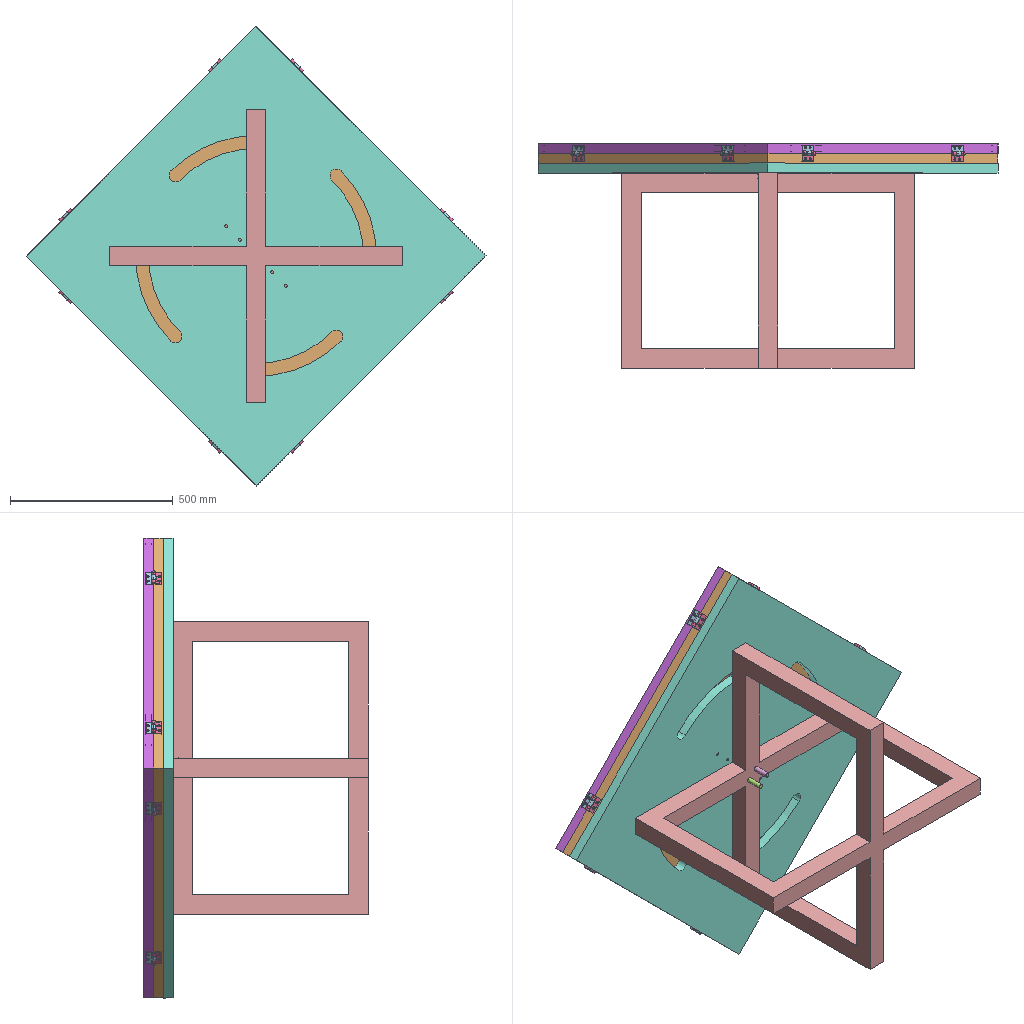Assembly | SolidWorks | 14 different items | 55 placed | box 1414 x 690 x 1414 mm
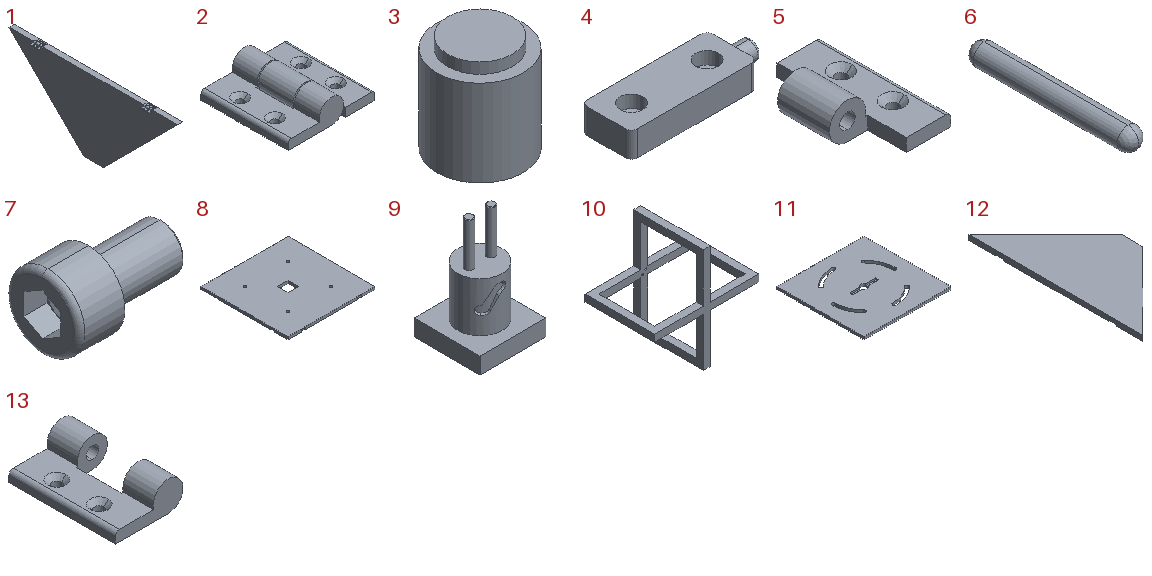Parts list (item | name | quantity | parent item | size | volume | features):
1 | (subassembly) | x4 | - | 55 x 1000 x 447 mm | 2719433 mm3 | -
2 | (subassembly) | x8 | in 1 | 50 x 50 x 14 mm | 16276 mm3 | -
3 | - | x4 | - | 40 x 40 x 45 mm | 53800 mm3 | features Extrusion 1, ICE 1
4 | - | x2 | - | 115 x 40 x 20 mm | 75193 mm3 | features Fillet 2, ICE 2, Extrusion 1
5 | - | x8 | in 2 | 32 x 50 x 14 mm | 6828 mm3 | features BaseBody 1
6 | - | x8 | in 2 | 6 x 46 x 6 mm | 1244 mm3 | features BaseBody 1
7 | - | x4 | - | 26 x 16 x 16 mm | 2933 mm3 | features Fillet 2, RevCut 2, Boss 1, Chamfer 1, Cut 1, Extrusion 1, LPattern 1
8 | - | x1 | - | 1000 x 1000 x 30 mm | 29440024 mm3 | features CirPattern 2, ICE 2, Extrusion 1, HoleWzd 1
9 | - | x1 | - | 120 x 120 x 200 mm | 904225 mm3 | features ICE 3, Chamfer 2, CirPattern 1, Emboss 1, Extrusion 1
10 | - | x1 | - | 900 x 600 x 900 mm | 19278601 mm3 | features ICE 2, Extrusion 1, HoleWzd 1
11 | - | x1 | - | 1000 x 1000 x 30 mm | 28197892 mm3 | features ICE 3, Extrusion 1, HoleWzd 1
12 | - | x4 | in 1 | 440 x 1000 x 30 mm | 2685666 mm3 | features Cut 1, Extrusion 1, HoleWzd 1, ICE 1, Shell 1
13 | - | x8 | in 2 | 32 x 50 x 14 mm | 8203 mm3 | features BaseBody 1
14 | cross recessed ctsk thread forming screw gb | x1 | - | - | - | -
Mates (type | each side: item.copy, entity, surface, feature):
In the top assembly
Concentric | 10.1 face cylinder Blind dowel hole 0 (size mm) | 9.1 face cylinder Boss-Extrude3 | 2 times
Concentric | 8.1 face cylinder Cut-Extrude1 | 3.1 face cylinder Boss-Extrude1
Concentric | 8.1 face cylinder Cut-Extrude1 | 3.2 face cylinder Boss-Extrude1
Concentric | 8.1 face cylinder Cut-Extrude1 | 3.3 face cylinder Boss-Extrude1
Concentric | 8.1 face cylinder Cut-Extrude1 | 3.4 face cylinder Boss-Extrude1
Coincident | 8.1 face plane Boss-Extrude1 | 3.4 face plane Boss-Extrude1
Coincident | 3.2 face plane Boss-Extrude1 | 3.4 face plane Boss-Extrude1
Coincident | 3.1 face plane Boss-Extrude1 | 3.4 face plane Boss-Extrude1
Coincident | 3.2 face plane Boss-Extrude1 | 3.3 face plane Boss-Extrude1
Parallel | 9.1 face plane Boss-Extrude1 | 8.1 face plane Boss-Extrude1
Coincident | 9.1 face plane Boss-Extrude1 | 8.1 face plane Boss-Extrude1 | 2 times
Concentric | 9.1 face cylinder Boss-Extrude2 | 11.1 face cylinder Cut-Extrude2
Coincident | 10.1 face plane Boss-Extrude1 | 11.1 face plane Boss-Extrude1
Coincident | 11.1 face plane Boss-Extrude1 | 8.1 face plane Boss-Extrude1
Concentric | 11.1 face cylinder M10 Tapped Hole1 | 4.1 face cylinder Boss-Extrude1 | 2 times
Coincident | 11.1 face plane Cut-Extrude3 | 4.1 face plane Boss-Extrude1
LimitDistanceDim | 9.1 face plane Boss-Extrude2 | 10.1 face plane Cut-Extrude1
LimitPlanarAngleDim | 11.1 face plane Boss-Extrude1 | 9.1 face plane Boss-Extrude1
Coincident | 8.1 face plane Cut-Extrude2 | 13.1 face plane Input 1
Coincident | 9.1 plane | 12.1 plane
Coincident | 8.1 face plane CirPattern1 | 13.2 face plane Input 1
Coincident | 9.1 plane | 12.2 plane
DistanceDim | 13.3 face plane Input 1 | 8.1 face plane Boss-Extrude1
Coincident | 8.1 face plane CirPattern1 | 13.4 face plane Input 1
Coincident | 8.1 face plane CirPattern1 | 13.5 face plane Input 1
Coincident | 9.1 plane | 12.3 plane
Coincident | 9.1 plane | 12.4 plane
DistanceDim | 13.6 face plane Input 1 | 8.1 face plane Boss-Extrude1
DistanceDim | 13.7 face plane Input 1 | 8.1 face plane Boss-Extrude1
LimitPlanarAngleDim | 12.2 face plane Boss-Extrude1 | 8.1 face plane Boss-Extrude1
DistanceDim | 13.8 face plane Input 1 | 8.1 face plane Boss-Extrude1
LimitPlanarAngleDim | 8.1 face plane Boss-Extrude1 | 12.1 face plane Boss-Extrude1
LimitPlanarAngleDim | 12.4 face plane Boss-Extrude1 | 8.1 face plane Boss-Extrude1
LimitPlanarAngleDim | 12.3 face plane Boss-Extrude1 | 8.1 face plane Boss-Extrude1
Coincident | 11.1 face plane Cut-Extrude3 | 4.2 face plane Boss-Extrude1
Concentric | 11.1 face cylinder M10 Tapped Hole1 | 4.2 face cylinder Cut-Extrude1
Concentric | 11.1 face cylinder M10 Tapped Hole1 | 4.2 edge
Concentric | 4.2 face cylinder Boss-Extrude1 | 7.1 face cylinder BaseBody
Coincident | 4.2 face plane Cut-Extrude1 | 7.1 face plane BaseHead
Concentric | 4.2 face cylinder Boss-Extrude1 | 7.2 face cylinder BaseBody
Coincident | 4.2 face plane Cut-Extrude1 | 7.2 face plane BaseHead
Concentric | 4.1 face cylinder Boss-Extrude1 | 7.3 face cylinder BaseBody
Coincident | 4.1 face plane Cut-Extrude1 | 7.3 face plane BaseHead
Concentric | 4.1 face cylinder Boss-Extrude1 | 7.4 face cylinder BaseBody
Coincident | 4.1 face plane Cut-Extrude1 | 7.4 face plane BaseHead
In subassembly 1
DistanceDim | 5.1 face plane Input 1 | 12.5 face plane Boss-Extrude1
DistanceDim | 5.1 face plane Input 1 | 12.5 edge
Coincident | 5.1 face plane Input 1 | 5.2 face plane Input 1
DistanceDim | 5.2 face plane Input 1 | 12.5 edge
Coincident | 5.1 face plane Input 1 | 12.5 face plane Cut-Extrude2
Coincident | 12.5 face plane Cut-Extrude2 | 5.2 face plane Input 1
In subassembly 2
Concentric | 13.9 face cylinder Input 1 | 6.1 face cylinder Input 1
Concentric | 13.9 face cylinder Input 1 | 5.3 face cylinder Input 1
Width | 5.3 face plane Input 1 | 5.3 face plane Input 1 | 13.9 face plane Input 1 | 13.9 face plane Input 1
Symmetric | 13.9 face plane Input 1 | 13.9 face plane Input 1 | 6.1 plane